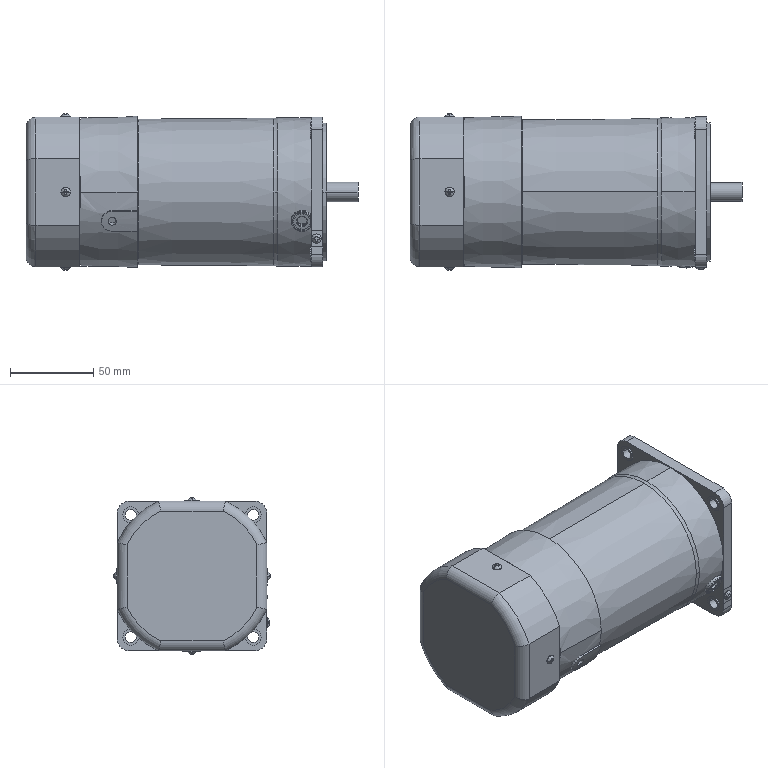Part | STEP file | S9R90G_ECE | 1 solid | 305 faces | box 199.4 x 93.897 x 93.895 mm | volume 1139593 mm3 | plane 152 | cylinder 99 | torus 27 | cone 16 | spline 10 | sphere 1 | commonest cylinder face diameters 5.6 x10 10 x9 3 x8 3.5 x8 6.5 x8 9.5 x8